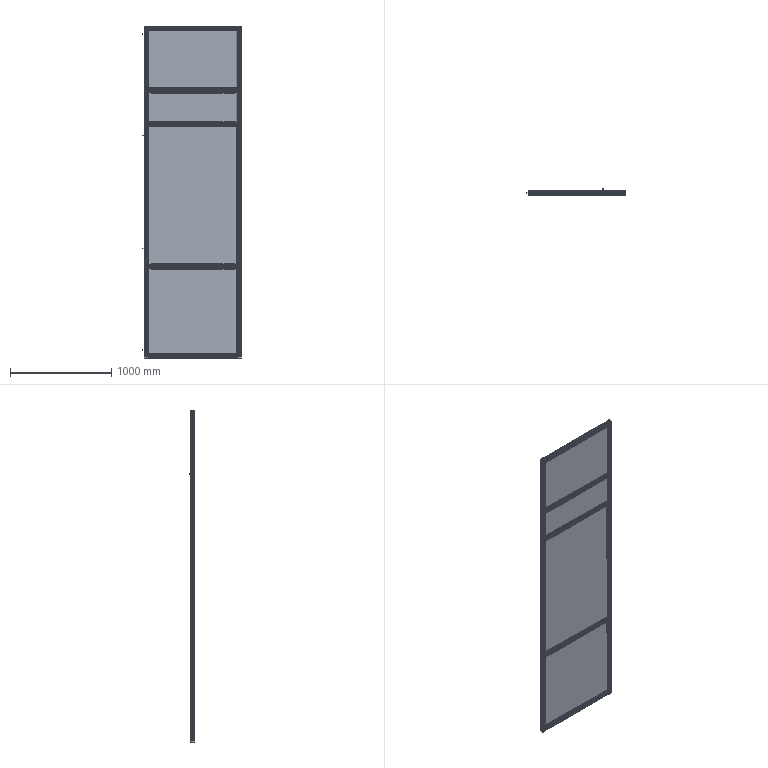Part | SolidWorks | 112 solids | 5225 faces | volume 21498613 mm3 | plane 3609 | cylinder 1348 | cone 220 | spline 48 | commonest cylinder face diameters 0.562 x200 6.8 x181 8 x88 2 x82 11 x72 19 x60